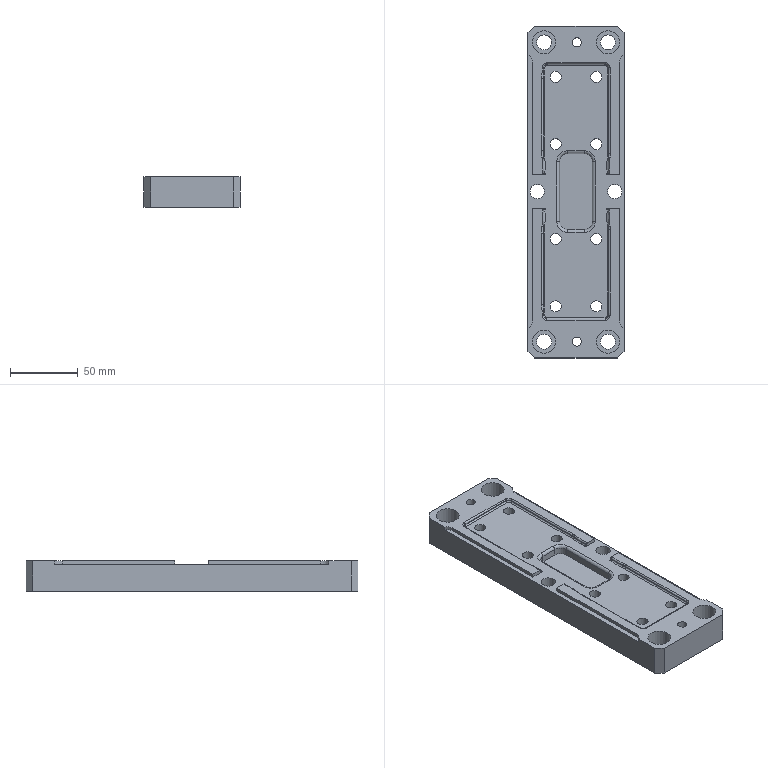Part | STEP file | 1_id114_x_t | 1 solid | 158 faces | box 71 x 245 x 22.4 mm | volume 320775 mm3 | cylinder 68 | plane 38 | torus 32 | spline 16 | other 4 | commonest cylinder face diameters 2 x18 3 x8 8.2 x8 4 x4 6 x4 11 x4